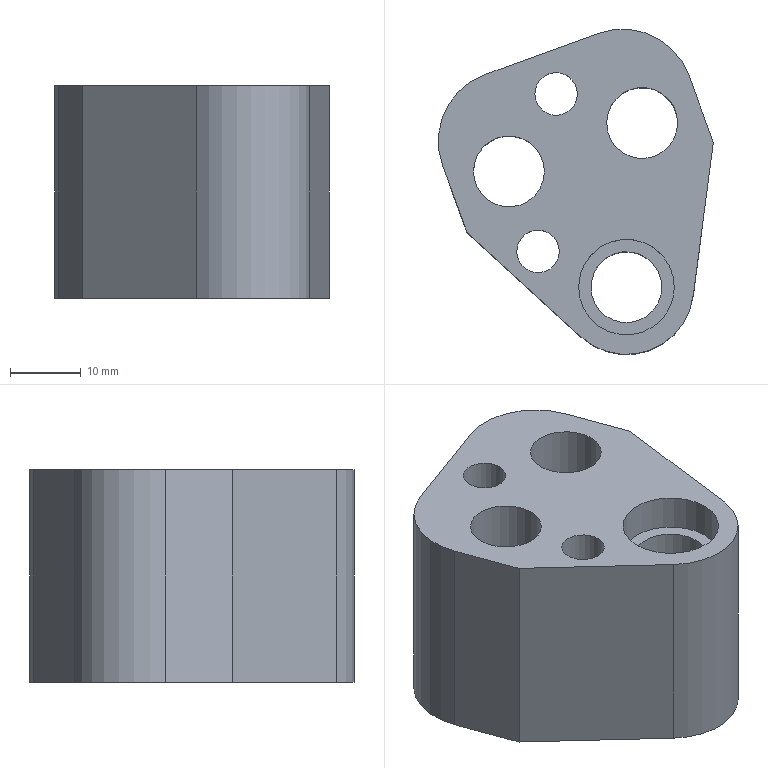Part | NX | features solid 2 | 1 solid | 25 faces | box 38.792 x 45.899 x 30 mm | volume 26942 mm3 | cylinder 13 | plane 12 | commonest cylinder face diameters 10 x3 6 x2 8 x2 14 x2 20 x2 13.5 x1
STEP:
#1=CARTESIAN_POINT('',(-707.064,-400.76,60.));
#2=VERTEX_POINT('',#1);
#3=CARTESIAN_POINT('',(-708.432,-397.001,60.));
#4=DIRECTION('',(0.,0.,1.));
#5=DIRECTION('',(0.342,-0.9397,0.));
#6=AXIS2_PLACEMENT_3D('',#3,#4,#5);
#7=CIRCLE('',#6,4.);
#8=EDGE_CURVE('',#2,#2,#7,.F.);
#9=ORIENTED_EDGE('',*,*,#8,.F.);
#10=EDGE_LOOP('',(#9));
#11=FACE_BOUND('',#10,.T.);
#12=CARTESIAN_POINT('',(-717.487,-401.361,60.));
#13=VERTEX_POINT('',#12);
#14=CARTESIAN_POINT('',(-715.093,-407.939,60.));
#15=DIRECTION('',(0.,0.,-1.));
#16=DIRECTION('',(-0.342,0.9397,0.));
#17=AXIS2_PLACEMENT_3D('',#14,#15,#16);
#18=CIRCLE('',#17,7.);
#19=EDGE_CURVE('',#13,#13,#18,.T.);
#20=ORIENTED_EDGE('',*,*,#19,.F.);
#21=EDGE_LOOP('',(#20));
#22=FACE_BOUND('',#21,.T.);
#23=CARTESIAN_POINT('',(-698.693,-394.52,60.));
#24=VERTEX_POINT('',#23);
#25=CARTESIAN_POINT('',(-696.299,-401.098,60.));
#26=DIRECTION('',(0.,0.,-1.));
#27=DIRECTION('',(-0.342,0.9397,0.));
#28=AXIS2_PLACEMENT_3D('',#25,#26,#27);
#29=CIRCLE('',#28,7.);
#30=EDGE_CURVE('',#24,#24,#29,.T.);
#31=ORIENTED_EDGE('',*,*,#30,.F.);
#32=EDGE_LOOP('',(#31));
#33=FACE_BOUND('',#32,.T.);
#34=CARTESIAN_POINT('',(-696.803,-428.95,60.));
#35=VERTEX_POINT('',#34);
#36=CARTESIAN_POINT('',(-698.513,-424.252,60.));
#37=DIRECTION('',(0.,0.,1.));
#38=DIRECTION('',(0.342,-0.9397,0.));
#39=AXIS2_PLACEMENT_3D('',#36,#37,#38);
#40=CIRCLE('',#39,5.);
#41=EDGE_CURVE('',#35,#35,#40,.T.);
#42=ORIENTED_EDGE('',*,*,#41,.T.);
#43=EDGE_LOOP('',(#42));
#44=FACE_BOUND('',#43,.T.);
#45=CARTESIAN_POINT('',(-689.094,-425.485,60.));
#46=VERTEX_POINT('',#45);
#47=CARTESIAN_POINT('',(-686.259,-403.829,60.));
#48=VERTEX_POINT('',#47);
#49=CARTESIAN_POINT('',(-689.094,-425.485,60.));
#50=DIRECTION('',(0.1298,0.9915,0.));
#51=VECTOR('',#50,1000.);
#52=LINE('',#49,#51);
#53=EDGE_CURVE('',#46,#48,#52,.T.);
#54=ORIENTED_EDGE('',*,*,#53,.F.);
#55=CARTESIAN_POINT('',(-704.937,-431.251,60.));
#56=VERTEX_POINT('',#55);
#57=CARTESIAN_POINT('',(-698.513,-424.252,60.));
#58=DIRECTION('',(0.,0.,-1.));
#59=DIRECTION('',(-0.342,0.9397,0.));
#60=AXIS2_PLACEMENT_3D('',#57,#58,#59);
#61=CIRCLE('',#60,9.5);
#62=EDGE_CURVE('',#46,#56,#61,.T.);
#63=ORIENTED_EDGE('',*,*,#62,.T.);
#64=CARTESIAN_POINT('',(-721.028,-416.484,60.));
#65=VERTEX_POINT('',#64);
#66=CARTESIAN_POINT('',(-704.937,-431.251,60.));
#67=DIRECTION('',(-0.7368,0.6761,0.));
#68=VECTOR('',#67,1000.);
#69=LINE('',#66,#68);
#70=EDGE_CURVE('',#56,#65,#69,.T.);
#71=ORIENTED_EDGE('',*,*,#70,.T.);
#72=CARTESIAN_POINT('',(-724.448,-407.087,60.));
#73=VERTEX_POINT('',#72);
#74=CARTESIAN_POINT('',(-721.028,-416.484,60.));
#75=DIRECTION('',(-0.342,0.9397,0.));
#76=VECTOR('',#75,1000.);
#77=LINE('',#74,#76);
#78=EDGE_CURVE('',#65,#73,#77,.T.);
#79=ORIENTED_EDGE('',*,*,#78,.T.);
#80=CARTESIAN_POINT('',(-718.472,-394.27,60.));
#81=VERTEX_POINT('',#80);
#82=CARTESIAN_POINT('',(-715.051,-403.667,60.));
#83=DIRECTION('',(0.,0.,-1.));
#84=DIRECTION('',(-0.342,0.9397,0.));
#85=AXIS2_PLACEMENT_3D('',#82,#83,#84);
#86=CIRCLE('',#85,10.);
#87=EDGE_CURVE('',#73,#81,#86,.T.);
#88=ORIENTED_EDGE('',*,*,#87,.T.);
#89=CARTESIAN_POINT('',(-702.497,-388.456,60.));
#90=VERTEX_POINT('',#89);
#91=CARTESIAN_POINT('',(-702.497,-388.456,60.));
#92=DIRECTION('',(-0.9397,-0.342,0.));
#93=VECTOR('',#92,1000.);
#94=LINE('',#91,#93);
#95=EDGE_CURVE('',#90,#81,#94,.T.);
#96=ORIENTED_EDGE('',*,*,#95,.F.);
#97=CARTESIAN_POINT('',(-689.68,-394.432,60.));
#98=VERTEX_POINT('',#97);
#99=CARTESIAN_POINT('',(-699.077,-397.852,60.));
#100=DIRECTION('',(0.,0.,-1.));
#101=DIRECTION('',(-0.342,0.9397,0.));
#102=AXIS2_PLACEMENT_3D('',#99,#100,#101);
#103=CIRCLE('',#102,10.);
#104=EDGE_CURVE('',#90,#98,#103,.T.);
#105=ORIENTED_EDGE('',*,*,#104,.T.);
#106=CARTESIAN_POINT('',(-686.259,-403.829,60.));
#107=DIRECTION('',(-0.342,0.9397,0.));
#108=VECTOR('',#107,1000.);
#109=LINE('',#106,#108);
#110=EDGE_CURVE('',#48,#98,#109,.T.);
#111=ORIENTED_EDGE('',*,*,#110,.F.);
#112=EDGE_LOOP('',(#54,#63,#71,#79,#88,#96,#105,#111));
#113=FACE_BOUND('',#112,.T.);
#114=CARTESIAN_POINT('',(-709.62,-422.974,60.));
#115=VERTEX_POINT('',#114);
#116=CARTESIAN_POINT('',(-710.989,-419.215,60.));
#117=DIRECTION('',(0.,0.,1.));
#118=DIRECTION('',(0.342,-0.9397,0.));
#119=AXIS2_PLACEMENT_3D('',#116,#117,#118);
#120=CIRCLE('',#119,4.);
#121=EDGE_CURVE('',#115,#115,#120,.F.);
#122=ORIENTED_EDGE('',*,*,#121,.F.);
#123=EDGE_LOOP('',(#122));
#124=FACE_BOUND('',#123,.T.);
#125=CARTESIAN_POINT('',(-699.077,-397.852,60.));
#126=DIRECTION('',(0.,0.,-1.));
#127=DIRECTION('',(-0.342,0.9397,0.));
#128=AXIS2_PLACEMENT_3D('',#125,#126,#127);
#129=PLANE('',#128);
#130=ADVANCED_FACE('',(#11,#22,#33,#44,#113,#124),#129,.T.);
#131=CARTESIAN_POINT('',(-709.458,-394.182,90.));
#132=VERTEX_POINT('',#131);
#133=CARTESIAN_POINT('',(-708.432,-397.001,90.));
#134=DIRECTION('',(0.,0.,-1.));
#135=DIRECTION('',(-0.342,0.9397,0.));
#136=AXIS2_PLACEMENT_3D('',#133,#134,#135);
#137=CIRCLE('',#136,3.);
#138=EDGE_CURVE('',#132,#132,#137,.T.);
#139=ORIENTED_EDGE('',*,*,#138,.F.);
#140=EDGE_LOOP('',(#139));
#141=FACE_BOUND('',#140,.T.);
#142=CARTESIAN_POINT('',(-709.458,-394.182,80.));
#143=VERTEX_POINT('',#142);
#144=CARTESIAN_POINT('',(-708.432,-397.001,80.));
#145=DIRECTION('',(0.,0.,-1.));
#146=DIRECTION('',(-0.342,0.9397,0.));
#147=AXIS2_PLACEMENT_3D('',#144,#145,#146);
#148=CIRCLE('',#147,3.);
#149=EDGE_CURVE('',#143,#143,#148,.T.);
#150=ORIENTED_EDGE('',*,*,#149,.T.);
#151=EDGE_LOOP('',(#150));
#152=FACE_BOUND('',#151,.T.);
#153=CARTESIAN_POINT('',(-708.432,-397.001,60.));
#154=DIRECTION('',(0.,0.,1.));
#155=DIRECTION('',(0.342,-0.9397,0.));
#156=AXIS2_PLACEMENT_3D('',#153,#154,#155);
#157=CYLINDRICAL_SURFACE('',#156,3.);
#158=ADVANCED_FACE('',(#141,#152),#157,.F.);
#159=CARTESIAN_POINT('',(-716.803,-403.24,90.));
#160=VERTEX_POINT('',#159);
#161=CARTESIAN_POINT('',(-715.093,-407.939,90.));
#162=DIRECTION('',(0.,0.,-1.));
#163=DIRECTION('',(-0.342,0.9397,0.));
#164=AXIS2_PLACEMENT_3D('',#161,#162,#163);
#165=CIRCLE('',#164,5.);
#166=EDGE_CURVE('',#160,#160,#165,.T.);
#167=ORIENTED_EDGE('',*,*,#166,.F.);
#168=EDGE_LOOP('',(#167));
#169=FACE_BOUND('',#168,.T.);
#170=CARTESIAN_POINT('',(-716.803,-403.24,70.));
#171=VERTEX_POINT('',#170);
#172=CARTESIAN_POINT('',(-715.093,-407.939,70.));
#173=DIRECTION('',(0.,0.,-1.));
#174=DIRECTION('',(-0.342,0.9397,0.));
#175=AXIS2_PLACEMENT_3D('',#172,#173,#174);
#176=CIRCLE('',#175,5.);
#177=EDGE_CURVE('',#171,#171,#176,.T.);
#178=ORIENTED_EDGE('',*,*,#177,.T.);
#179=EDGE_LOOP('',(#178));
#180=FACE_BOUND('',#179,.T.);
#181=CARTESIAN_POINT('',(-715.093,-407.939,60.));
#182=DIRECTION('',(0.,0.,1.));
#183=DIRECTION('',(0.342,-0.9397,0.));
#184=AXIS2_PLACEMENT_3D('',#181,#182,#183);
#185=CYLINDRICAL_SURFACE('',#184,5.);
#186=ADVANCED_FACE('',(#169,#180),#185,.F.);
#187=CARTESIAN_POINT('',(-698.009,-396.4,90.));
#188=VERTEX_POINT('',#187);
#189=CARTESIAN_POINT('',(-696.299,-401.098,90.));
#190=DIRECTION('',(0.,0.,-1.));
#191=DIRECTION('',(-0.342,0.9397,0.));
#192=AXIS2_PLACEMENT_3D('',#189,#190,#191);
#193=CIRCLE('',#192,5.);
#194=EDGE_CURVE('',#188,#188,#193,.T.);
#195=ORIENTED_EDGE('',*,*,#194,.F.);
#196=EDGE_LOOP('',(#195));
#197=FACE_BOUND('',#196,.T.);
#198=CARTESIAN_POINT('',(-698.009,-396.4,70.));
#199=VERTEX_POINT('',#198);
#200=CARTESIAN_POINT('',(-696.299,-401.098,70.));
#201=DIRECTION('',(0.,0.,-1.));
#202=DIRECTION('',(-0.342,0.9397,0.));
#203=AXIS2_PLACEMENT_3D('',#200,#201,#202);
#204=CIRCLE('',#203,5.);
#205=EDGE_CURVE('',#199,#199,#204,.T.);
#206=ORIENTED_EDGE('',*,*,#205,.T.);
#207=EDGE_LOOP('',(#206));
#208=FACE_BOUND('',#207,.T.);
#209=CARTESIAN_POINT('',(-696.299,-401.098,60.));
#210=DIRECTION('',(0.,0.,1.));
#211=DIRECTION('',(0.342,-0.9397,0.));
#212=AXIS2_PLACEMENT_3D('',#209,#210,#211);
#213=CYLINDRICAL_SURFACE('',#212,5.);
#214=ADVANCED_FACE('',(#197,#208),#213,.F.);
#215=CARTESIAN_POINT('',(-712.015,-416.396,90.));
#216=VERTEX_POINT('',#215);
#217=CARTESIAN_POINT('',(-710.989,-419.215,90.));
#218=DIRECTION('',(0.,0.,-1.));
#219=DIRECTION('',(-0.342,0.9397,0.));
#220=AXIS2_PLACEMENT_3D('',#217,#218,#219);
#221=CIRCLE('',#220,3.);
#222=EDGE_CURVE('',#216,#216,#221,.T.);
#223=ORIENTED_EDGE('',*,*,#222,.T.);
#224=EDGE_LOOP('',(#223));
#225=FACE_BOUND('',#224,.T.);
#226=ORIENTED_EDGE('',*,*,#166,.T.);
#227=EDGE_LOOP('',(#226));
#228=FACE_BOUND('',#227,.T.);
#229=CARTESIAN_POINT('',(-689.094,-425.485,90.));
#230=VERTEX_POINT('',#229);
#231=CARTESIAN_POINT('',(-686.259,-403.829,90.));
#232=VERTEX_POINT('',#231);
#233=CARTESIAN_POINT('',(-689.094,-425.485,90.));
#234=DIRECTION('',(0.1298,0.9915,0.));
#235=VECTOR('',#234,1000.);
#236=LINE('',#233,#235);
#237=EDGE_CURVE('',#230,#232,#236,.T.);
#238=ORIENTED_EDGE('',*,*,#237,.T.);
#239=CARTESIAN_POINT('',(-689.68,-394.432,90.));
#240=VERTEX_POINT('',#239);
#241=CARTESIAN_POINT('',(-686.259,-403.829,90.));
#242=DIRECTION('',(-0.342,0.9397,0.));
#243=VECTOR('',#242,1000.);
#244=LINE('',#241,#243);
#245=EDGE_CURVE('',#232,#240,#244,.T.);
#246=ORIENTED_EDGE('',*,*,#245,.T.);
#247=CARTESIAN_POINT('',(-702.497,-388.456,90.));
#248=VERTEX_POINT('',#247);
#249=CARTESIAN_POINT('',(-699.077,-397.852,90.));
#250=DIRECTION('',(0.,0.,-1.));
#251=DIRECTION('',(-0.342,0.9397,0.));
#252=AXIS2_PLACEMENT_3D('',#249,#250,#251);
#253=CIRCLE('',#252,10.);
#254=EDGE_CURVE('',#248,#240,#253,.T.);
#255=ORIENTED_EDGE('',*,*,#254,.F.);
#256=CARTESIAN_POINT('',(-718.472,-394.27,90.));
#257=VERTEX_POINT('',#256);
#258=CARTESIAN_POINT('',(-702.497,-388.456,90.));
#259=DIRECTION('',(-0.9397,-0.342,0.));
#260=VECTOR('',#259,1000.);
#261=LINE('',#258,#260);
#262=EDGE_CURVE('',#248,#257,#261,.T.);
#263=ORIENTED_EDGE('',*,*,#262,.T.);
#264=CARTESIAN_POINT('',(-724.448,-407.087,90.));
#265=VERTEX_POINT('',#264);
#266=CARTESIAN_POINT('',(-715.051,-403.667,90.));
#267=DIRECTION('',(0.,0.,-1.));
#268=DIRECTION('',(-0.342,0.9397,0.));
#269=AXIS2_PLACEMENT_3D('',#266,#267,#268);
#270=CIRCLE('',#269,10.);
#271=EDGE_CURVE('',#265,#257,#270,.T.);
#272=ORIENTED_EDGE('',*,*,#271,.F.);
#273=CARTESIAN_POINT('',(-721.028,-416.484,90.));
#274=VERTEX_POINT('',#273);
#275=CARTESIAN_POINT('',(-721.028,-416.484,90.));
#276=DIRECTION('',(-0.342,0.9397,0.));
#277=VECTOR('',#276,1000.);
#278=LINE('',#275,#277);
#279=EDGE_CURVE('',#274,#265,#278,.T.);
#280=ORIENTED_EDGE('',*,*,#279,.F.);
#281=CARTESIAN_POINT('',(-704.937,-431.251,90.));
#282=VERTEX_POINT('',#281);
#283=CARTESIAN_POINT('',(-704.937,-431.251,90.));
#284=DIRECTION('',(-0.7368,0.6761,0.));
#285=VECTOR('',#284,1000.);
#286=LINE('',#283,#285);
#287=EDGE_CURVE('',#282,#274,#286,.T.);
#288=ORIENTED_EDGE('',*,*,#287,.F.);
#289=CARTESIAN_POINT('',(-698.513,-424.252,90.));
#290=DIRECTION('',(0.,0.,-1.));
#291=DIRECTION('',(-0.342,0.9397,0.));
#292=AXIS2_PLACEMENT_3D('',#289,#290,#291);
#293=CIRCLE('',#292,9.5);
#294=EDGE_CURVE('',#230,#282,#293,.T.);
#295=ORIENTED_EDGE('',*,*,#294,.F.);
#296=EDGE_LOOP('',(#238,#246,#255,#263,#272,#280,#288,#295));
#297=FACE_BOUND('',#296,.T.);
#298=CARTESIAN_POINT('',(-700.822,-417.909,90.));
#299=VERTEX_POINT('',#298);
#300=CARTESIAN_POINT('',(-698.513,-424.252,90.));
#301=DIRECTION('',(0.,0.,-1.));
#302=DIRECTION('',(-0.342,0.9397,0.));
#303=AXIS2_PLACEMENT_3D('',#300,#301,#302);
#304=CIRCLE('',#303,6.75);
#305=EDGE_CURVE('',#299,#299,#304,.T.);
#306=ORIENTED_EDGE('',*,*,#305,.T.);
#307=EDGE_LOOP('',(#306));
#308=FACE_BOUND('',#307,.T.);
#309=ORIENTED_EDGE('',*,*,#194,.T.);
#310=EDGE_LOOP('',(#309));
#311=FACE_BOUND('',#310,.T.);
#312=ORIENTED_EDGE('',*,*,#138,.T.);
#313=EDGE_LOOP('',(#312));
#314=FACE_BOUND('',#313,.T.);
#315=CARTESIAN_POINT('',(-699.077,-397.852,90.));
#316=DIRECTION('',(0.,0.,-1.));
#317=DIRECTION('',(-0.342,0.9397,0.));
#318=AXIS2_PLACEMENT_3D('',#315,#316,#317);
#319=PLANE('',#318);
#320=ADVANCED_FACE('',(#225,#228,#297,#308,#311,#314),#319,.F.);
#321=ORIENTED_EDGE('',*,*,#237,.F.);
#322=CARTESIAN_POINT('',(-689.094,-425.485,60.));
#323=DIRECTION('',(0.,0.,1.));
#324=VECTOR('',#323,1000.);
#325=LINE('',#322,#324);
#326=EDGE_CURVE('',#46,#230,#325,.T.);
#327=ORIENTED_EDGE('',*,*,#326,.F.);
#328=ORIENTED_EDGE('',*,*,#53,.T.);
#329=CARTESIAN_POINT('',(-686.259,-403.829,60.));
#330=DIRECTION('',(0.,0.,1.));
#331=VECTOR('',#330,1000.);
#332=LINE('',#329,#331);
#333=EDGE_CURVE('',#48,#232,#332,.T.);
#334=ORIENTED_EDGE('',*,*,#333,.T.);
#335=EDGE_LOOP('',(#321,#327,#328,#334));
#336=FACE_BOUND('',#335,.T.);
#337=CARTESIAN_POINT('',(-689.094,-425.485,60.));
#338=DIRECTION('',(0.9915,-0.1298,0.));
#339=DIRECTION('',(0.1298,0.9915,0.));
#340=AXIS2_PLACEMENT_3D('',#337,#338,#339);
#341=PLANE('',#340);
#342=ADVANCED_FACE('',(#336),#341,.T.);
#343=ORIENTED_EDGE('',*,*,#245,.F.);
#344=ORIENTED_EDGE('',*,*,#333,.F.);
#345=ORIENTED_EDGE('',*,*,#110,.T.);
#346=CARTESIAN_POINT('',(-689.68,-394.432,60.));
#347=DIRECTION('',(0.,0.,1.));
#348=VECTOR('',#347,1000.);
#349=LINE('',#346,#348);
#350=EDGE_CURVE('',#98,#240,#349,.T.);
#351=ORIENTED_EDGE('',*,*,#350,.T.);
#352=EDGE_LOOP('',(#343,#344,#345,#351));
#353=FACE_BOUND('',#352,.T.);
#354=CARTESIAN_POINT('',(-686.259,-403.829,60.));
#355=DIRECTION('',(0.9397,0.342,0.));
#356=DIRECTION('',(-0.342,0.9397,0.));
#357=AXIS2_PLACEMENT_3D('',#354,#355,#356);
#358=PLANE('',#357);
#359=ADVANCED_FACE('',(#353),#358,.T.);
#360=ORIENTED_EDGE('',*,*,#254,.T.);
#361=ORIENTED_EDGE('',*,*,#350,.F.);
#362=ORIENTED_EDGE('',*,*,#104,.F.);
#363=CARTESIAN_POINT('',(-702.497,-388.456,60.));
#364=DIRECTION('',(0.,0.,1.));
#365=VECTOR('',#364,1000.);
#366=LINE('',#363,#365);
#367=EDGE_CURVE('',#90,#248,#366,.T.);
#368=ORIENTED_EDGE('',*,*,#367,.T.);
#369=EDGE_LOOP('',(#360,#361,#362,#368));
#370=FACE_BOUND('',#369,.T.);
#371=CARTESIAN_POINT('',(-699.077,-397.852,60.));
#372=DIRECTION('',(0.,0.,1.));
#373=DIRECTION('',(0.342,-0.9397,0.));
#374=AXIS2_PLACEMENT_3D('',#371,#372,#373);
#375=CYLINDRICAL_SURFACE('',#374,10.);
#376=ADVANCED_FACE('',(#370),#375,.T.);
#377=ORIENTED_EDGE('',*,*,#262,.F.);
#378=ORIENTED_EDGE('',*,*,#367,.F.);
#379=ORIENTED_EDGE('',*,*,#95,.T.);
#380=CARTESIAN_POINT('',(-718.472,-394.27,60.));
#381=DIRECTION('',(0.,0.,1.));
#382=VECTOR('',#381,1000.);
#383=LINE('',#380,#382);
#384=EDGE_CURVE('',#81,#257,#383,.T.);
#385=ORIENTED_EDGE('',*,*,#384,.T.);
#386=EDGE_LOOP('',(#377,#378,#379,#385));
#387=FACE_BOUND('',#386,.T.);
#388=CARTESIAN_POINT('',(-702.497,-388.456,60.));
#389=DIRECTION('',(-0.342,0.9397,0.));
#390=DIRECTION('',(-0.9397,-0.342,0.));
#391=AXIS2_PLACEMENT_3D('',#388,#389,#390);
#392=PLANE('',#391);
#393=ADVANCED_FACE('',(#387),#392,.T.);
#394=ORIENTED_EDGE('',*,*,#271,.T.);
#395=ORIENTED_EDGE('',*,*,#384,.F.);
#396=ORIENTED_EDGE('',*,*,#87,.F.);
#397=CARTESIAN_POINT('',(-724.448,-407.087,60.));
#398=DIRECTION('',(0.,0.,1.));
#399=VECTOR('',#398,1000.);
#400=LINE('',#397,#399);
#401=EDGE_CURVE('',#73,#265,#400,.T.);
#402=ORIENTED_EDGE('',*,*,#401,.T.);
#403=EDGE_LOOP('',(#394,#395,#396,#402));
#404=FACE_BOUND('',#403,.T.);
#405=CARTESIAN_POINT('',(-715.051,-403.667,60.));
#406=DIRECTION('',(0.,0.,1.));
#407=DIRECTION('',(0.342,-0.9397,0.));
#408=AXIS2_PLACEMENT_3D('',#405,#406,#407);
#409=CYLINDRICAL_SURFACE('',#408,10.);
#410=ADVANCED_FACE('',(#404),#409,.T.);
#411=ORIENTED_EDGE('',*,*,#279,.T.);
#412=ORIENTED_EDGE('',*,*,#401,.F.);
#413=ORIENTED_EDGE('',*,*,#78,.F.);
#414=CARTESIAN_POINT('',(-721.028,-416.484,60.));
#415=DIRECTION('',(0.,0.,1.));
#416=VECTOR('',#415,1000.);
#417=LINE('',#414,#416);
#418=EDGE_CURVE('',#65,#274,#417,.T.);
#419=ORIENTED_EDGE('',*,*,#418,.T.);
#420=EDGE_LOOP('',(#411,#412,#413,#419));
#421=FACE_BOUND('',#420,.T.);
#422=CARTESIAN_POINT('',(-721.028,-416.484,60.));
#423=DIRECTION('',(0.9397,0.342,0.));
#424=DIRECTION('',(-0.342,0.9397,0.));
#425=AXIS2_PLACEMENT_3D('',#422,#423,#424);
#426=PLANE('',#425);
#427=ADVANCED_FACE('',(#421),#426,.F.);
#428=ORIENTED_EDGE('',*,*,#287,.T.);
#429=ORIENTED_EDGE('',*,*,#418,.F.);
#430=ORIENTED_EDGE('',*,*,#70,.F.);
#431=CARTESIAN_POINT('',(-704.937,-431.251,60.));
#432=DIRECTION('',(0.,0.,1.));
#433=VECTOR('',#432,1000.);
#434=LINE('',#431,#433);
#435=EDGE_CURVE('',#56,#282,#434,.T.);
#436=ORIENTED_EDGE('',*,*,#435,.T.);
#437=EDGE_LOOP('',(#428,#429,#430,#436));
#438=FACE_BOUND('',#437,.T.);
#439=CARTESIAN_POINT('',(-704.937,-431.251,60.));
#440=DIRECTION('',(0.6761,0.7368,0.));
#441=DIRECTION('',(-0.7368,0.6761,0.));
#442=AXIS2_PLACEMENT_3D('',#439,#440,#441);
#443=PLANE('',#442);
#444=ADVANCED_FACE('',(#438),#443,.F.);
#445=ORIENTED_EDGE('',*,*,#294,.T.);
#446=ORIENTED_EDGE('',*,*,#435,.F.);
#447=ORIENTED_EDGE('',*,*,#62,.F.);
#448=ORIENTED_EDGE('',*,*,#326,.T.);
#449=EDGE_LOOP('',(#445,#446,#447,#448));
#450=FACE_BOUND('',#449,.T.);
#451=CARTESIAN_POINT('',(-698.513,-424.252,60.));
#452=DIRECTION('',(0.,0.,1.));
#453=DIRECTION('',(0.342,-0.9397,0.));
#454=AXIS2_PLACEMENT_3D('',#451,#452,#453);
#455=CYLINDRICAL_SURFACE('',#454,9.5);
#456=ADVANCED_FACE('',(#450),#455,.T.);
#457=CARTESIAN_POINT('',(-700.224,-419.553,85.));
#458=VERTEX_POINT('',#457);
#459=CARTESIAN_POINT('',(-698.513,-424.252,85.));
#460=DIRECTION('',(0.,0.,-1.));
#461=DIRECTION('',(-0.342,0.9397,0.));
#462=AXIS2_PLACEMENT_3D('',#459,#460,#461);
#463=CIRCLE('',#462,5.);
#464=EDGE_CURVE('',#458,#458,#463,.F.);
#465=ORIENTED_EDGE('',*,*,#464,.T.);
#466=EDGE_LOOP('',(#465));
#467=FACE_BOUND('',#466,.T.);
#468=ORIENTED_EDGE('',*,*,#41,.F.);
#469=EDGE_LOOP('',(#468));
#470=FACE_BOUND('',#469,.T.);
#471=CARTESIAN_POINT('',(-698.513,-424.252,60.));
#472=DIRECTION('',(0.,0.,1.));
#473=DIRECTION('',(0.342,-0.9397,0.));
#474=AXIS2_PLACEMENT_3D('',#471,#472,#473);
#475=CYLINDRICAL_SURFACE('',#474,5.);
#476=ADVANCED_FACE('',(#467,#470),#475,.F.);
#477=CARTESIAN_POINT('',(-700.822,-417.909,85.));
#478=VERTEX_POINT('',#477);
#479=CARTESIAN_POINT('',(-698.513,-424.252,85.));
#480=DIRECTION('',(0.,0.,-1.));
#481=DIRECTION('',(-0.342,0.9397,0.));
#482=AXIS2_PLACEMENT_3D('',#479,#480,#481);
#483=CIRCLE('',#482,6.75);
#484=EDGE_CURVE('',#478,#478,#483,.T.);
#485=ORIENTED_EDGE('',*,*,#484,.F.);
#486=EDGE_LOOP('',(#485));
#487=FACE_BOUND('',#486,.T.);
#488=ORIENTED_EDGE('',*,*,#464,.F.);
#489=EDGE_LOOP('',(#488));
#490=FACE_BOUND('',#489,.T.);
#491=CARTESIAN_POINT('',(-698.513,-424.252,85.));
#492=DIRECTION('',(0.,0.,-1.));
#493=DIRECTION('',(-0.342,0.9397,0.));
#494=AXIS2_PLACEMENT_3D('',#491,#492,#493);
#495=PLANE('',#494);
#496=ADVANCED_FACE('',(#487,#490),#495,.F.);
#497=ORIENTED_EDGE('',*,*,#484,.T.);
#498=EDGE_LOOP('',(#497));
#499=FACE_BOUND('',#498,.T.);
#500=ORIENTED_EDGE('',*,*,#305,.F.);
#501=EDGE_LOOP('',(#500));
#502=FACE_BOUND('',#501,.T.);
#503=CARTESIAN_POINT('',(-698.513,-424.252,85.));
#504=DIRECTION('',(0.,0.,1.));
#505=DIRECTION('',(0.342,-0.9397,0.));
#506=AXIS2_PLACEMENT_3D('',#503,#504,#505);
#507=CYLINDRICAL_SURFACE('',#506,6.75);
#508=ADVANCED_FACE('',(#499,#502),#507,.F.);
#509=CARTESIAN_POINT('',(-712.015,-416.396,80.));
#510=VERTEX_POINT('',#509);
#511=CARTESIAN_POINT('',(-710.989,-419.215,80.));
#512=DIRECTION('',(0.,0.,-1.));
#513=DIRECTION('',(-0.342,0.9397,0.));
#514=AXIS2_PLACEMENT_3D('',#511,#512,#513);
#515=CIRCLE('',#514,3.);
#516=EDGE_CURVE('',#510,#510,#515,.T.);
#517=ORIENTED_EDGE('',*,*,#516,.T.);
#518=EDGE_LOOP('',(#517));
#519=FACE_BOUND('',#518,.T.);
#520=ORIENTED_EDGE('',*,*,#222,.F.);
#521=EDGE_LOOP('',(#520));
#522=FACE_BOUND('',#521,.T.);
#523=CARTESIAN_POINT('',(-710.989,-419.215,60.));
#524=DIRECTION('',(0.,0.,1.));
#525=DIRECTION('',(0.342,-0.9397,0.));
#526=AXIS2_PLACEMENT_3D('',#523,#524,#525);
#527=CYLINDRICAL_SURFACE('',#526,3.);
#528=ADVANCED_FACE('',(#519,#522),#527,.F.);
#529=CARTESIAN_POINT('',(-698.693,-394.52,70.));
#530=VERTEX_POINT('',#529);
#531=CARTESIAN_POINT('',(-696.299,-401.098,70.));
#532=DIRECTION('',(0.,0.,-1.));
#533=DIRECTION('',(-0.342,0.9397,0.));
#534=AXIS2_PLACEMENT_3D('',#531,#532,#533);
#535=CIRCLE('',#534,7.);
#536=EDGE_CURVE('',#530,#530,#535,.T.);
#537=ORIENTED_EDGE('',*,*,#536,.F.);
#538=EDGE_LOOP('',(#537));
#539=FACE_BOUND('',#538,.T.);
#540=ORIENTED_EDGE('',*,*,#30,.T.);
#541=EDGE_LOOP('',(#540));
#542=FACE_BOUND('',#541,.T.);
#543=CARTESIAN_POINT('',(-696.299,-401.098,70.));
#544=DIRECTION('',(0.,0.,-1.));
#545=DIRECTION('',(-0.342,0.9397,0.));
#546=AXIS2_PLACEMENT_3D('',#543,#544,#545);
#547=CYLINDRICAL_SURFACE('',#546,7.);
#548=ADVANCED_FACE('',(#539,#542),#547,.F.);
#549=ORIENTED_EDGE('',*,*,#205,.F.);
#550=EDGE_LOOP('',(#549));
#551=FACE_BOUND('',#550,.T.);
#552=ORIENTED_EDGE('',*,*,#536,.T.);
#553=EDGE_LOOP('',(#552));
#554=FACE_BOUND('',#553,.T.);
#555=CARTESIAN_POINT('',(-696.299,-401.098,70.));
#556=DIRECTION('',(0.,0.,-1.));
#557=DIRECTION('',(-0.342,0.9397,0.));
#558=AXIS2_PLACEMENT_3D('',#555,#556,#557);
#559=PLANE('',#558);
#560=ADVANCED_FACE('',(#551,#554),#559,.T.);
#561=CARTESIAN_POINT('',(-717.487,-401.361,70.));
#562=VERTEX_POINT('',#561);
#563=CARTESIAN_POINT('',(-715.093,-407.939,70.));
#564=DIRECTION('',(0.,0.,-1.));
#565=DIRECTION('',(-0.342,0.9397,0.));
#566=AXIS2_PLACEMENT_3D('',#563,#564,#565);
#567=CIRCLE('',#566,7.);
#568=EDGE_CURVE('',#562,#562,#567,.T.);
#569=ORIENTED_EDGE('',*,*,#568,.F.);
#570=EDGE_LOOP('',(#569));
#571=FACE_BOUND('',#570,.T.);
#572=ORIENTED_EDGE('',*,*,#19,.T.);
#573=EDGE_LOOP('',(#572));
#574=FACE_BOUND('',#573,.T.);
#575=CARTESIAN_POINT('',(-715.093,-407.939,70.));
#576=DIRECTION('',(0.,0.,-1.));
#577=DIRECTION('',(-0.342,0.9397,0.));
#578=AXIS2_PLACEMENT_3D('',#575,#576,#577);
#579=CYLINDRICAL_SURFACE('',#578,7.);
#580=ADVANCED_FACE('',(#571,#574),#579,.F.);
#581=ORIENTED_EDGE('',*,*,#177,.F.);
#582=EDGE_LOOP('',(#581));
#583=FACE_BOUND('',#582,.T.);
#584=ORIENTED_EDGE('',*,*,#568,.T.);
#585=EDGE_LOOP('',(#584));
#586=FACE_BOUND('',#585,.T.);
#587=CARTESIAN_POINT('',(-715.093,-407.939,70.));
#588=DIRECTION('',(0.,0.,-1.));
#589=DIRECTION('',(-0.342,0.9397,0.));
#590=AXIS2_PLACEMENT_3D('',#587,#588,#589);
#591=PLANE('',#590);
#592=ADVANCED_FACE('',(#583,#586),#591,.T.);
#593=ORIENTED_EDGE('',*,*,#149,.F.);
#594=EDGE_LOOP('',(#593));
#595=FACE_BOUND('',#594,.T.);
#596=CARTESIAN_POINT('',(-707.064,-400.76,80.));
#597=VERTEX_POINT('',#596);
#598=CARTESIAN_POINT('',(-708.432,-397.001,80.));
#599=DIRECTION('',(0.,0.,1.));
#600=DIRECTION('',(0.342,-0.9397,0.));
#601=AXIS2_PLACEMENT_3D('',#598,#599,#600);
#602=CIRCLE('',#601,4.);
#603=EDGE_CURVE('',#597,#597,#602,.F.);
#604=ORIENTED_EDGE('',*,*,#603,.T.);
#605=EDGE_LOOP('',(#604));
#606=FACE_BOUND('',#605,.T.);
#607=CARTESIAN_POINT('',(-708.432,-397.001,80.));
#608=DIRECTION('',(0.,0.,1.));
#609=DIRECTION('',(0.342,-0.9397,0.));
#610=AXIS2_PLACEMENT_3D('',#607,#608,#609);
#611=PLANE('',#610);
#612=ADVANCED_FACE('',(#595,#606),#611,.F.);
#613=ORIENTED_EDGE('',*,*,#603,.F.);
#614=EDGE_LOOP('',(#613));
#615=FACE_BOUND('',#614,.T.);
#616=ORIENTED_EDGE('',*,*,#8,.T.);
#617=EDGE_LOOP('',(#616));
#618=FACE_BOUND('',#617,.T.);
#619=CARTESIAN_POINT('',(-708.432,-397.001,60.));
#620=DIRECTION('',(0.,0.,1.));
#621=DIRECTION('',(0.342,-0.9397,0.));
#622=AXIS2_PLACEMENT_3D('',#619,#620,#621);
#623=CYLINDRICAL_SURFACE('',#622,4.);
#624=ADVANCED_FACE('',(#615,#618),#623,.F.);
#625=ORIENTED_EDGE('',*,*,#516,.F.);
#626=EDGE_LOOP('',(#625));
#627=FACE_BOUND('',#626,.T.);
#628=CARTESIAN_POINT('',(-709.62,-422.974,80.));
#629=VERTEX_POINT('',#628);
#630=CARTESIAN_POINT('',(-710.989,-419.215,80.));
#631=DIRECTION('',(0.,0.,1.));
#632=DIRECTION('',(0.342,-0.9397,0.));
#633=AXIS2_PLACEMENT_3D('',#630,#631,#632);
#634=CIRCLE('',#633,4.);
#635=EDGE_CURVE('',#629,#629,#634,.F.);
#636=ORIENTED_EDGE('',*,*,#635,.T.);
#637=EDGE_LOOP('',(#636));
#638=FACE_BOUND('',#637,.T.);
#639=CARTESIAN_POINT('',(-710.989,-419.215,80.));
#640=DIRECTION('',(0.,0.,1.));
#641=DIRECTION('',(0.342,-0.9397,0.));
#642=AXIS2_PLACEMENT_3D('',#639,#640,#641);
#643=PLANE('',#642);
#644=ADVANCED_FACE('',(#627,#638),#643,.F.);
#645=ORIENTED_EDGE('',*,*,#635,.F.);
#646=EDGE_LOOP('',(#645));
#647=FACE_BOUND('',#646,.T.);
#648=ORIENTED_EDGE('',*,*,#121,.T.);
#649=EDGE_LOOP('',(#648));
#650=FACE_BOUND('',#649,.T.);
#651=CARTESIAN_POINT('',(-710.989,-419.215,60.));
#652=DIRECTION('',(0.,0.,1.));
#653=DIRECTION('',(0.342,-0.9397,0.));
#654=AXIS2_PLACEMENT_3D('',#651,#652,#653);
#655=CYLINDRICAL_SURFACE('',#654,4.);
#656=ADVANCED_FACE('',(#647,#650),#655,.F.);
#657=CLOSED_SHELL('',(#130,#158,#186,#214,#320,#342,#359,#376,#393,#410,#427,#444,#456,#476,#496,#508,#528,#548,#560,#580,#592,#612,#624,#644,#656));
#658=MANIFOLD_SOLID_BREP('',#657);
#659=(LENGTH_UNIT()NAMED_UNIT(*)SI_UNIT(.MILLI.,.METRE.));
#660=UNCERTAINTY_MEASURE_WITH_UNIT(LENGTH_MEASURE(0.00001),#659,'','');
#661=(NAMED_UNIT(*)PLANE_ANGLE_UNIT()SI_UNIT($,.RADIAN.));
#662=(NAMED_UNIT(*)SI_UNIT($,.STERADIAN.)SOLID_ANGLE_UNIT());
#663=(GEOMETRIC_REPRESENTATION_CONTEXT(3)GLOBAL_UNCERTAINTY_ASSIGNED_CONTEXT((#660))GLOBAL_UNIT_ASSIGNED_CONTEXT((#659,#661,#662))REPRESENTATION_CONTEXT('',''));
#664=ADVANCED_BREP_SHAPE_REPRESENTATION('',(#658),#663);